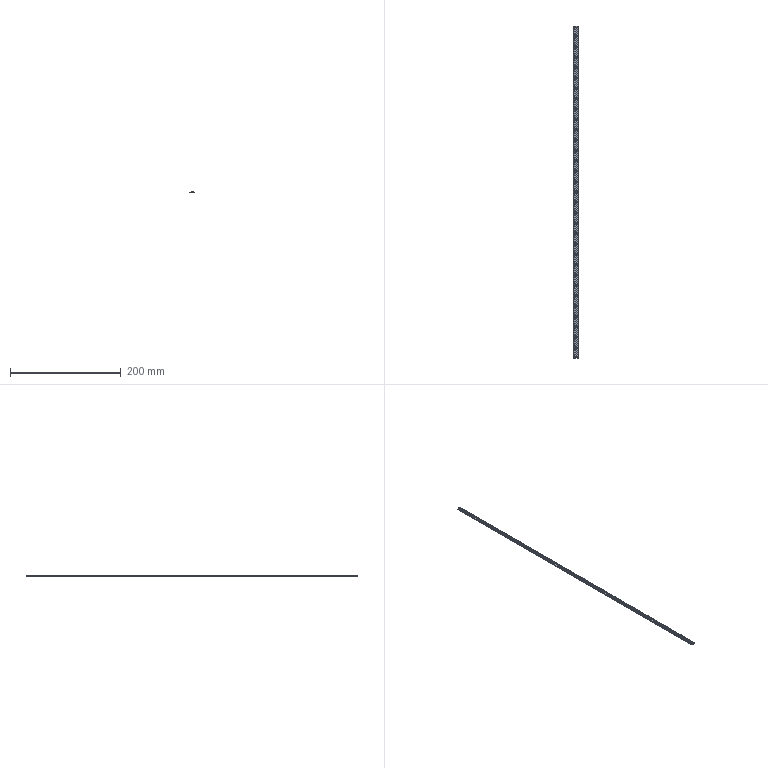Part | SolidWorks | features ICE 4, LPattern 4, Extrusion 1 | 1 solid | 2108 faces | box 8 x 600 x 1.5 mm | volume 1218 mm3 | plane 1509 | cylinder 599 | commonest cylinder face diameters 1.5 x300 0.8 x299